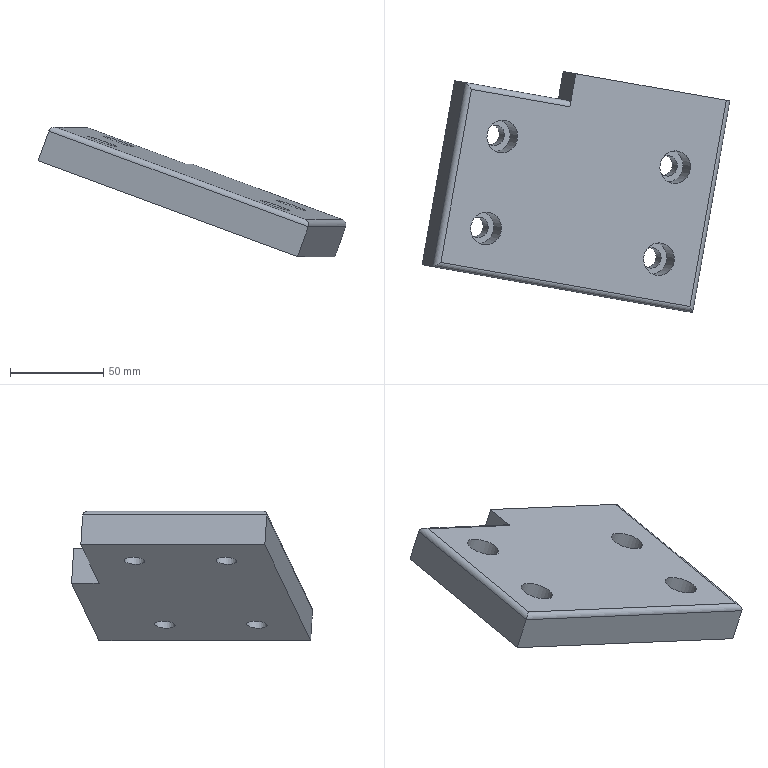Part | NX | features solid 2 | 1 solid | 24 faces | box 164.686 x 128.953 x 69.252 mm | volume 311600 mm3 | plane 12 | cylinder 12 | commonest cylinder face diameters 6 x4 11 x4 17.5 x4
STEP:
#1=CARTESIAN_POINT('',(-964.598,583.981,-183.949));
#2=VERTEX_POINT('',#1);
#3=CARTESIAN_POINT('',(-1020.123,593.771,-163.428));
#4=VERTEX_POINT('',#3);
#5=CARTESIAN_POINT('',(-834.947,561.12,-231.866));
#6=DIRECTION('',(-0.9254,0.1632,0.342));
#7=VECTOR('',#6,1000.);
#8=LINE('',#5,#7);
#9=EDGE_CURVE('',#2,#4,#8,.T.);
#10=ORIENTED_EDGE('',*,*,#9,.F.);
#11=CARTESIAN_POINT('',(-970.324,584.991,-199.924));
#12=VERTEX_POINT('',#11);
#13=CARTESIAN_POINT('',(-963.554,583.797,-181.036));
#14=DIRECTION('',(-0.3368,0.05939,-0.9397));
#15=VECTOR('',#14,1000.);
#16=LINE('',#13,#15);
#17=EDGE_CURVE('',#2,#12,#16,.T.);
#18=ORIENTED_EDGE('',*,*,#17,.T.);
#19=CARTESIAN_POINT('',(-1025.849,594.781,-179.402));
#20=VERTEX_POINT('',#19);
#21=CARTESIAN_POINT('',(-840.581,562.113,-247.875));
#22=DIRECTION('',(-0.9254,0.1632,0.342));
#23=VECTOR('',#22,1000.);
#24=LINE('',#21,#23);
#25=EDGE_CURVE('',#12,#20,#24,.T.);
#26=ORIENTED_EDGE('',*,*,#25,.T.);
#27=CARTESIAN_POINT('',(-1019.079,593.587,-160.515));
#28=DIRECTION('',(-0.3368,0.05939,-0.9397));
#29=VECTOR('',#28,1000.);
#30=LINE('',#27,#29);
#31=EDGE_CURVE('',#4,#20,#30,.T.);
#32=ORIENTED_EDGE('',*,*,#31,.F.);
#33=EDGE_LOOP('',(#10,#18,#26,#32));
#34=FACE_BOUND('',#33,.T.);
#35=CARTESIAN_POINT('',(-833.903,560.936,-228.953));
#36=DIRECTION('',(0.1736,0.9848,0.));
#37=DIRECTION('',(-0.9254,0.1632,0.342));
#38=AXIS2_PLACEMENT_3D('',#35,#36,#37);
#39=PLANE('',#38);
#40=ADVANCED_FACE('',(#34),#39,.T.);
#41=CARTESIAN_POINT('',(-898.675,470.814,-214.731));
#42=VERTEX_POINT('',#41);
#43=CARTESIAN_POINT('',(-878.706,584.067,-214.731));
#44=VERTEX_POINT('',#43);
#45=CARTESIAN_POINT('',(-880.625,573.185,-214.731));
#46=DIRECTION('',(-0.1736,-0.9848,0.));
#47=VECTOR('',#46,1000.);
#48=LINE('',#45,#47);
#49=EDGE_CURVE('',#42,#44,#48,.F.);
#50=ORIENTED_EDGE('',*,*,#49,.T.);
#51=CARTESIAN_POINT('',(-880.472,584.379,-210.886));
#52=VERTEX_POINT('',#51);
#53=CARTESIAN_POINT('',(-881.482,584.557,-213.705));
#54=DIRECTION('',(0.1736,0.9848,0.));
#55=DIRECTION('',(-0.9848,0.1736,0.));
#56=AXIS2_PLACEMENT_3D('',#53,#54,#55);
#57=CIRCLE('',#56,3.);
#58=EDGE_CURVE('',#44,#52,#57,.F.);
#59=ORIENTED_EDGE('',*,*,#58,.T.);
#60=CARTESIAN_POINT('',(-899.92,474.08,-210.886));
#61=VERTEX_POINT('',#60);
#62=CARTESIAN_POINT('',(-902.629,458.717,-210.886));
#63=DIRECTION('',(-0.1736,-0.9848,0.));
#64=VECTOR('',#63,1000.);
#65=LINE('',#62,#64);
#66=EDGE_CURVE('',#52,#61,#65,.T.);
#67=ORIENTED_EDGE('',*,*,#66,.T.);
#68=CARTESIAN_POINT('',(-900.931,474.258,-213.705));
#69=DIRECTION('',(0.7772,0.581,-0.2418));
#70=DIRECTION('',(0.5316,-0.8117,-0.2418));
#71=AXIS2_PLACEMENT_3D('',#68,#69,#70);
#72=ELLIPSE('',#71,4.243,3.);
#73=EDGE_CURVE('',#61,#42,#72,.T.);
#74=ORIENTED_EDGE('',*,*,#73,.T.);
#75=EDGE_LOOP('',(#50,#59,#67,#74));
#76=FACE_BOUND('',#75,.T.);
#77=CARTESIAN_POINT('',(-903.639,458.895,-213.705));
#78=DIRECTION('',(-0.1736,-0.9848,0.));
#79=DIRECTION('',(-0.9848,0.1736,0.));
#80=AXIS2_PLACEMENT_3D('',#77,#78,#79);
#81=CYLINDRICAL_SURFACE('',#80,3.);
#82=ADVANCED_FACE('',(#76),#81,.T.);
#83=CARTESIAN_POINT('',(-1016.857,590.149,-161.635));
#84=VERTEX_POINT('',#83);
#85=CARTESIAN_POINT('',(-964.108,580.848,-181.13));
#86=VERTEX_POINT('',#85);
#87=CARTESIAN_POINT('',(-834.365,557.971,-229.081));
#88=DIRECTION('',(-0.9254,0.1632,0.342));
#89=VECTOR('',#88,1000.);
#90=LINE('',#87,#89);
#91=EDGE_CURVE('',#84,#86,#90,.F.);
#92=ORIENTED_EDGE('',*,*,#91,.T.);
#93=CARTESIAN_POINT('',(-965.119,581.026,-183.949));
#94=DIRECTION('',(0.9254,-0.1632,-0.342));
#95=DIRECTION('',(-0.3467,0.,-0.938));
#96=AXIS2_PLACEMENT_3D('',#93,#94,#95);
#97=CIRCLE('',#96,3.);
#98=EDGE_CURVE('',#86,#2,#97,.F.);
#99=ORIENTED_EDGE('',*,*,#98,.T.);
#100=ORIENTED_EDGE('',*,*,#9,.T.);
#101=CARTESIAN_POINT('',(-1017.868,590.328,-164.454));
#102=DIRECTION('',(0.7772,0.581,-0.2418));
#103=DIRECTION('',(-0.5316,0.8117,0.2418));
#104=AXIS2_PLACEMENT_3D('',#101,#102,#103);
#105=ELLIPSE('',#104,4.243,3.);
#106=EDGE_CURVE('',#4,#84,#105,.T.);
#107=ORIENTED_EDGE('',*,*,#106,.T.);
#108=EDGE_LOOP('',(#92,#99,#100,#107));
#109=FACE_BOUND('',#108,.T.);
#110=CARTESIAN_POINT('',(-835.468,558.166,-231.866));
#111=DIRECTION('',(-0.9254,0.1632,0.342));
#112=DIRECTION('',(0.3368,-0.05939,0.9397));
#113=AXIS2_PLACEMENT_3D('',#110,#111,#112);
#114=CYLINDRICAL_SURFACE('',#113,3.);
#115=ADVANCED_FACE('',(#109),#114,.T.);
#116=CARTESIAN_POINT('',(-960.983,598.575,-181.13));
#117=VERTEX_POINT('',#116);
#118=CARTESIAN_POINT('',(-963.587,583.803,-181.13));
#119=DIRECTION('',(-0.1736,-0.9848,0.));
#120=VECTOR('',#119,1000.);
#121=LINE('',#118,#120);
#122=EDGE_CURVE('',#86,#117,#121,.F.);
#123=ORIENTED_EDGE('',*,*,#122,.F.);
#124=ORIENTED_EDGE('',*,*,#91,.F.);
#125=CARTESIAN_POINT('',(-1033.18,497.577,-161.635));
#126=VERTEX_POINT('',#125);
#127=CARTESIAN_POINT('',(-1035.889,482.214,-161.635));
#128=DIRECTION('',(-0.1736,-0.9848,0.));
#129=VECTOR('',#128,1000.);
#130=LINE('',#127,#129);
#131=EDGE_CURVE('',#126,#84,#130,.F.);
#132=ORIENTED_EDGE('',*,*,#131,.F.);
#133=CARTESIAN_POINT('',(-850.688,465.399,-229.081));
#134=DIRECTION('',(-0.9254,0.1632,0.342));
#135=VECTOR('',#134,1000.);
#136=LINE('',#133,#135);
#137=EDGE_CURVE('',#61,#126,#136,.T.);
#138=ORIENTED_EDGE('',*,*,#137,.F.);
#139=ORIENTED_EDGE('',*,*,#66,.F.);
#140=CARTESIAN_POINT('',(-831.332,575.714,-229.047));
#141=DIRECTION('',(0.9254,-0.1632,-0.342));
#142=VECTOR('',#141,1000.);
#143=LINE('',#140,#142);
#144=EDGE_CURVE('',#52,#117,#143,.F.);
#145=ORIENTED_EDGE('',*,*,#144,.T.);
#146=EDGE_LOOP('',(#123,#124,#132,#138,#139,#145));
#147=FACE_BOUND('',#146,.T.);
#148=CARTESIAN_POINT('',(-924.556,500.764,-200.368));
#149=VERTEX_POINT('',#148);
#150=CARTESIAN_POINT('',(-916.459,499.336,-203.361));
#151=DIRECTION('',(0.3368,-0.05939,0.9397));
#152=DIRECTION('',(-0.9254,0.1632,0.342));
#153=AXIS2_PLACEMENT_3D('',#150,#151,#152);
#154=CIRCLE('',#153,8.75);
#155=EDGE_CURVE('',#149,#149,#154,.T.);
#156=ORIENTED_EDGE('',*,*,#155,.F.);
#157=EDGE_LOOP('',(#156));
#158=FACE_BOUND('',#157,.T.);
#159=CARTESIAN_POINT('',(-915.874,550.004,-200.368));
#160=VERTEX_POINT('',#159);
#161=CARTESIAN_POINT('',(-907.777,548.576,-203.361));
#162=DIRECTION('',(0.3368,-0.05939,0.9397));
#163=DIRECTION('',(-0.9254,0.1632,0.342));
#164=AXIS2_PLACEMENT_3D('',#161,#162,#163);
#165=CIRCLE('',#164,8.75);
#166=EDGE_CURVE('',#160,#160,#165,.T.);
#167=ORIENTED_EDGE('',*,*,#166,.F.);
#168=EDGE_LOOP('',(#167));
#169=FACE_BOUND('',#168,.T.);
#170=CARTESIAN_POINT('',(-992.221,563.466,-172.152));
#171=VERTEX_POINT('',#170);
#172=CARTESIAN_POINT('',(-1000.318,564.894,-169.159));
#173=DIRECTION('',(-0.3368,0.05939,-0.9397));
#174=DIRECTION('',(0.9254,-0.1632,-0.342));
#175=AXIS2_PLACEMENT_3D('',#172,#173,#174);
#176=CIRCLE('',#175,8.75);
#177=EDGE_CURVE('',#171,#171,#176,.F.);
#178=ORIENTED_EDGE('',*,*,#177,.F.);
#179=EDGE_LOOP('',(#178));
#180=FACE_BOUND('',#179,.T.);
#181=CARTESIAN_POINT('',(-1000.903,514.226,-172.152));
#182=VERTEX_POINT('',#181);
#183=CARTESIAN_POINT('',(-1009.001,515.653,-169.159));
#184=DIRECTION('',(-0.3368,0.05939,-0.9397));
#185=DIRECTION('',(0.9254,-0.1632,-0.342));
#186=AXIS2_PLACEMENT_3D('',#183,#184,#185);
#187=CIRCLE('',#186,8.75);
#188=EDGE_CURVE('',#182,#182,#187,.F.);
#189=ORIENTED_EDGE('',*,*,#188,.F.);
#190=EDGE_LOOP('',(#189));
#191=FACE_BOUND('',#190,.T.);
#192=CARTESIAN_POINT('',(-853.397,450.036,-229.081));
#193=DIRECTION('',(0.3368,-0.05939,0.9397));
#194=DIRECTION('',(-0.9254,0.1632,0.342));
#195=AXIS2_PLACEMENT_3D('',#192,#193,#194);
#196=PLANE('',#195);
#197=ADVANCED_FACE('',(#147,#158,#169,#180,#191),#196,.T.);
#198=CARTESIAN_POINT('',(-884.432,585.077,-230.705));
#199=VERTEX_POINT('',#198);
#200=CARTESIAN_POINT('',(-877.662,583.883,-211.818));
#201=DIRECTION('',(0.3368,-0.05939,0.9397));
#202=VECTOR('',#201,1000.);
#203=LINE('',#200,#202);
#204=EDGE_CURVE('',#199,#44,#203,.T.);
#205=ORIENTED_EDGE('',*,*,#204,.T.);
#206=ORIENTED_EDGE('',*,*,#49,.F.);
#207=CARTESIAN_POINT('',(-904.401,471.824,-230.705));
#208=VERTEX_POINT('',#207);
#209=CARTESIAN_POINT('',(-904.772,471.889,-231.739));
#210=DIRECTION('',(0.3368,-0.05939,0.9397));
#211=VECTOR('',#210,1000.);
#212=LINE('',#209,#211);
#213=EDGE_CURVE('',#208,#42,#212,.T.);
#214=ORIENTED_EDGE('',*,*,#213,.F.);
#215=CARTESIAN_POINT('',(-906.572,459.514,-230.705));
#216=DIRECTION('',(0.1736,0.9848,0.));
#217=VECTOR('',#216,1000.);
#218=LINE('',#215,#217);
#219=EDGE_CURVE('',#208,#199,#218,.T.);
#220=ORIENTED_EDGE('',*,*,#219,.T.);
#221=EDGE_LOOP('',(#205,#206,#214,#220));
#222=FACE_BOUND('',#221,.T.);
#223=CARTESIAN_POINT('',(-886.721,574.26,-231.739));
#224=DIRECTION('',(0.9254,-0.1632,-0.342));
#225=DIRECTION('',(-0.1736,-0.9848,0.));
#226=AXIS2_PLACEMENT_3D('',#223,#224,#225);
#227=PLANE('',#226);
#228=ADVANCED_FACE('',(#222),#227,.T.);
#229=ORIENTED_EDGE('',*,*,#25,.F.);
#230=CARTESIAN_POINT('',(-967.719,599.763,-199.924));
#231=VERTEX_POINT('',#230);
#232=CARTESIAN_POINT('',(-970.324,584.991,-199.924));
#233=DIRECTION('',(0.1736,0.9848,0.));
#234=VECTOR('',#233,1000.);
#235=LINE('',#232,#234);
#236=EDGE_CURVE('',#12,#231,#235,.T.);
#237=ORIENTED_EDGE('',*,*,#236,.T.);
#238=CARTESIAN_POINT('',(-837.976,576.885,-247.875));
#239=DIRECTION('',(-0.9254,0.1632,0.342));
#240=VECTOR('',#239,1000.);
#241=LINE('',#238,#240);
#242=EDGE_CURVE('',#199,#231,#241,.T.);
#243=ORIENTED_EDGE('',*,*,#242,.F.);
#244=ORIENTED_EDGE('',*,*,#219,.F.);
#245=CARTESIAN_POINT('',(-1043.214,496.3,-179.402));
#246=VERTEX_POINT('',#245);
#247=CARTESIAN_POINT('',(-857.945,463.633,-247.875));
#248=DIRECTION('',(0.9254,-0.1632,-0.342));
#249=VECTOR('',#248,1000.);
#250=LINE('',#247,#249);
#251=EDGE_CURVE('',#246,#208,#250,.T.);
#252=ORIENTED_EDGE('',*,*,#251,.F.);
#253=CARTESIAN_POINT('',(-1028.176,581.585,-179.402));
#254=DIRECTION('',(0.1736,0.9848,0.));
#255=VECTOR('',#254,1000.);
#256=LINE('',#253,#255);
#257=EDGE_CURVE('',#246,#20,#256,.T.);
#258=ORIENTED_EDGE('',*,*,#257,.T.);
#259=EDGE_LOOP('',(#229,#237,#243,#244,#252,#258));
#260=FACE_BOUND('',#259,.T.);
#261=CARTESIAN_POINT('',(-928.285,501.421,-220.274));
#262=VERTEX_POINT('',#261);
#263=CARTESIAN_POINT('',(-923.196,500.524,-222.155));
#264=DIRECTION('',(0.3368,-0.05939,0.9397));
#265=DIRECTION('',(-0.9254,0.1632,0.342));
#266=AXIS2_PLACEMENT_3D('',#263,#264,#265);
#267=CIRCLE('',#266,5.5);
#268=EDGE_CURVE('',#262,#262,#267,.T.);
#269=ORIENTED_EDGE('',*,*,#268,.T.);
#270=EDGE_LOOP('',(#269));
#271=FACE_BOUND('',#270,.T.);
#272=CARTESIAN_POINT('',(-919.603,550.661,-220.274));
#273=VERTEX_POINT('',#272);
#274=CARTESIAN_POINT('',(-914.513,549.764,-222.155));
#275=DIRECTION('',(0.3368,-0.05939,0.9397));
#276=DIRECTION('',(-0.9254,0.1632,0.342));
#277=AXIS2_PLACEMENT_3D('',#274,#275,#276);
#278=CIRCLE('',#277,5.5);
#279=EDGE_CURVE('',#273,#273,#278,.T.);
#280=ORIENTED_EDGE('',*,*,#279,.T.);
#281=EDGE_LOOP('',(#280));
#282=FACE_BOUND('',#281,.T.);
#283=CARTESIAN_POINT('',(-1012.145,566.979,-186.072));
#284=VERTEX_POINT('',#283);
#285=CARTESIAN_POINT('',(-1007.055,566.082,-187.953));
#286=DIRECTION('',(0.3368,-0.05939,0.9397));
#287=DIRECTION('',(-0.9254,0.1632,0.342));
#288=AXIS2_PLACEMENT_3D('',#285,#286,#287);
#289=CIRCLE('',#288,5.5);
#290=EDGE_CURVE('',#284,#284,#289,.T.);
#291=ORIENTED_EDGE('',*,*,#290,.T.);
#292=EDGE_LOOP('',(#291));
#293=FACE_BOUND('',#292,.T.);
#294=CARTESIAN_POINT('',(-1020.827,517.739,-186.072));
#295=VERTEX_POINT('',#294);
#296=CARTESIAN_POINT('',(-1015.737,516.841,-187.953));
#297=DIRECTION('',(0.3368,-0.05939,0.9397));
#298=DIRECTION('',(-0.9254,0.1632,0.342));
#299=AXIS2_PLACEMENT_3D('',#296,#297,#298);
#300=CIRCLE('',#299,5.5);
#301=EDGE_CURVE('',#295,#295,#300,.T.);
#302=ORIENTED_EDGE('',*,*,#301,.T.);
#303=EDGE_LOOP('',(#302));
#304=FACE_BOUND('',#303,.T.);
#305=CARTESIAN_POINT('',(-839.877,566.102,-247.875));
#306=DIRECTION('',(-0.3368,0.05939,-0.9397));
#307=DIRECTION('',(-0.9254,0.1632,0.342));
#308=AXIS2_PLACEMENT_3D('',#305,#306,#307);
#309=PLANE('',#308);
#310=ADVANCED_FACE('',(#260,#271,#282,#293,#304),#309,.T.);
#311=ORIENTED_EDGE('',*,*,#31,.T.);
#312=ORIENTED_EDGE('',*,*,#257,.F.);
#313=CARTESIAN_POINT('',(-1037.488,495.291,-163.428));
#314=VERTEX_POINT('',#313);
#315=CARTESIAN_POINT('',(-1036.444,495.107,-160.515));
#316=DIRECTION('',(-0.3368,0.05939,-0.9397));
#317=VECTOR('',#316,1000.);
#318=LINE('',#315,#317);
#319=EDGE_CURVE('',#314,#246,#318,.T.);
#320=ORIENTED_EDGE('',*,*,#319,.F.);
#321=CARTESIAN_POINT('',(-1022.45,580.575,-163.428));
#322=DIRECTION('',(-0.1736,-0.9848,0.));
#323=VECTOR('',#322,1000.);
#324=LINE('',#321,#323);
#325=EDGE_CURVE('',#4,#314,#324,.T.);
#326=ORIENTED_EDGE('',*,*,#325,.F.);
#327=EDGE_LOOP('',(#311,#312,#320,#326));
#328=FACE_BOUND('',#327,.T.);
#329=CARTESIAN_POINT('',(-1021.406,580.391,-160.515));
#330=DIRECTION('',(-0.9254,0.1632,0.342));
#331=DIRECTION('',(-0.1736,-0.9848,0.));
#332=AXIS2_PLACEMENT_3D('',#329,#330,#331);
#333=PLANE('',#332);
#334=ADVANCED_FACE('',(#328),#333,.T.);
#335=ORIENTED_EDGE('',*,*,#319,.T.);
#336=ORIENTED_EDGE('',*,*,#251,.T.);
#337=ORIENTED_EDGE('',*,*,#213,.T.);
#338=CARTESIAN_POINT('',(-845.464,461.432,-234.397));
#339=DIRECTION('',(-0.9254,0.1632,0.342));
#340=VECTOR('',#339,1000.);
#341=LINE('',#338,#340);
#342=EDGE_CURVE('',#314,#42,#341,.F.);
#343=ORIENTED_EDGE('',*,*,#342,.F.);
#344=EDGE_LOOP('',(#335,#336,#337,#343));
#345=FACE_BOUND('',#344,.T.);
#346=CARTESIAN_POINT('',(-851.527,462.501,-251.311));
#347=DIRECTION('',(-0.1736,-0.9848,0.));
#348=DIRECTION('',(-0.9254,0.1632,0.342));
#349=AXIS2_PLACEMENT_3D('',#346,#347,#348);
#350=PLANE('',#349);
#351=ADVANCED_FACE('',(#345),#350,.T.);
#352=ORIENTED_EDGE('',*,*,#268,.F.);
#353=EDGE_LOOP('',(#352));
#354=FACE_BOUND('',#353,.T.);
#355=CARTESIAN_POINT('',(-925.591,500.946,-212.756));
#356=VERTEX_POINT('',#355);
#357=CARTESIAN_POINT('',(-920.501,500.048,-214.637));
#358=DIRECTION('',(0.3368,-0.05939,0.9397));
#359=DIRECTION('',(-0.9254,0.1632,0.342));
#360=AXIS2_PLACEMENT_3D('',#357,#358,#359);
#361=CIRCLE('',#360,5.5);
#362=EDGE_CURVE('',#356,#356,#361,.T.);
#363=ORIENTED_EDGE('',*,*,#362,.T.);
#364=EDGE_LOOP('',(#363));
#365=FACE_BOUND('',#364,.T.);
#366=CARTESIAN_POINT('',(-933.3,502.305,-250.346));
#367=DIRECTION('',(-0.3368,0.05939,-0.9397));
#368=DIRECTION('',(-0.9254,0.1632,0.342));
#369=AXIS2_PLACEMENT_3D('',#366,#367,#368);
#370=CYLINDRICAL_SURFACE('',#369,5.5);
#371=ADVANCED_FACE('',(#354,#365),#370,.F.);
#372=ORIENTED_EDGE('',*,*,#362,.F.);
#373=EDGE_LOOP('',(#372));
#374=FACE_BOUND('',#373,.T.);
#375=CARTESIAN_POINT('',(-928.598,501.476,-211.645));
#376=VERTEX_POINT('',#375);
#377=CARTESIAN_POINT('',(-920.501,500.048,-214.637));
#378=DIRECTION('',(0.3368,-0.05939,0.9397));
#379=DIRECTION('',(-0.9254,0.1632,0.342));
#380=AXIS2_PLACEMENT_3D('',#377,#378,#379);
#381=CIRCLE('',#380,8.75);
#382=EDGE_CURVE('',#376,#376,#381,.T.);
#383=ORIENTED_EDGE('',*,*,#382,.T.);
#384=EDGE_LOOP('',(#383));
#385=FACE_BOUND('',#384,.T.);
#386=CARTESIAN_POINT('',(-872.146,503.707,-231.738));
#387=DIRECTION('',(-0.3368,0.05939,-0.9397));
#388=DIRECTION('',(-0.9254,0.1632,0.342));
#389=AXIS2_PLACEMENT_3D('',#386,#387,#388);
#390=PLANE('',#389);
#391=ADVANCED_FACE('',(#374,#385),#390,.F.);
#392=ORIENTED_EDGE('',*,*,#382,.F.);
#393=EDGE_LOOP('',(#392));
#394=FACE_BOUND('',#393,.T.);
#395=ORIENTED_EDGE('',*,*,#155,.T.);
#396=EDGE_LOOP('',(#395));
#397=FACE_BOUND('',#396,.T.);
#398=CARTESIAN_POINT('',(-916.459,499.336,-203.361));
#399=DIRECTION('',(-0.3368,0.05939,-0.9397));
#400=DIRECTION('',(-0.9254,0.1632,0.342));
#401=AXIS2_PLACEMENT_3D('',#398,#399,#400);
#402=CYLINDRICAL_SURFACE('',#401,8.75);
#403=ADVANCED_FACE('',(#394,#397),#402,.F.);
#404=ORIENTED_EDGE('',*,*,#279,.F.);
#405=EDGE_LOOP('',(#404));
#406=FACE_BOUND('',#405,.T.);
#407=CARTESIAN_POINT('',(-916.908,550.186,-212.756));
#408=VERTEX_POINT('',#407);
#409=CARTESIAN_POINT('',(-911.818,549.289,-214.637));
#410=DIRECTION('',(0.3368,-0.05939,0.9397));
#411=DIRECTION('',(-0.9254,0.1632,0.342));
#412=AXIS2_PLACEMENT_3D('',#409,#410,#411);
#413=CIRCLE('',#412,5.5);
#414=EDGE_CURVE('',#408,#408,#413,.T.);
#415=ORIENTED_EDGE('',*,*,#414,.T.);
#416=EDGE_LOOP('',(#415));
#417=FACE_BOUND('',#416,.T.);
#418=CARTESIAN_POINT('',(-924.618,551.546,-250.346));
#419=DIRECTION('',(-0.3368,0.05939,-0.9397));
#420=DIRECTION('',(-0.9254,0.1632,0.342));
#421=AXIS2_PLACEMENT_3D('',#418,#419,#420);
#422=CYLINDRICAL_SURFACE('',#421,5.5);
#423=ADVANCED_FACE('',(#406,#417),#422,.F.);
#424=ORIENTED_EDGE('',*,*,#414,.F.);
#425=EDGE_LOOP('',(#424));
#426=FACE_BOUND('',#425,.T.);
#427=CARTESIAN_POINT('',(-919.916,550.717,-211.645));
#428=VERTEX_POINT('',#427);
#429=CARTESIAN_POINT('',(-911.818,549.289,-214.637));
#430=DIRECTION('',(0.3368,-0.05939,0.9397));
#431=DIRECTION('',(-0.9254,0.1632,0.342));
#432=AXIS2_PLACEMENT_3D('',#429,#430,#431);
#433=CIRCLE('',#432,8.75);
#434=EDGE_CURVE('',#428,#428,#433,.T.);
#435=ORIENTED_EDGE('',*,*,#434,.T.);
#436=EDGE_LOOP('',(#435));
#437=FACE_BOUND('',#436,.T.);
#438=CARTESIAN_POINT('',(-867.805,528.328,-231.738));
#439=DIRECTION('',(-0.3368,0.05939,-0.9397));
#440=DIRECTION('',(-0.9254,0.1632,0.342));
#441=AXIS2_PLACEMENT_3D('',#438,#439,#440);
#442=PLANE('',#441);
#443=ADVANCED_FACE('',(#426,#437),#442,.F.);
#444=ORIENTED_EDGE('',*,*,#434,.F.);
#445=EDGE_LOOP('',(#444));
#446=FACE_BOUND('',#445,.T.);
#447=ORIENTED_EDGE('',*,*,#166,.T.);
#448=EDGE_LOOP('',(#447));
#449=FACE_BOUND('',#448,.T.);
#450=CARTESIAN_POINT('',(-907.777,548.576,-203.361));
#451=DIRECTION('',(-0.3368,0.05939,-0.9397));
#452=DIRECTION('',(-0.9254,0.1632,0.342));
#453=AXIS2_PLACEMENT_3D('',#450,#451,#452);
#454=CYLINDRICAL_SURFACE('',#453,8.75);
#455=ADVANCED_FACE('',(#446,#449),#454,.F.);
#456=ORIENTED_EDGE('',*,*,#290,.F.);
#457=EDGE_LOOP('',(#456));
#458=FACE_BOUND('',#457,.T.);
#459=CARTESIAN_POINT('',(-1009.45,566.504,-178.554));
#460=VERTEX_POINT('',#459);
#461=CARTESIAN_POINT('',(-1004.36,565.606,-180.435));
#462=DIRECTION('',(0.3368,-0.05939,0.9397));
#463=DIRECTION('',(-0.9254,0.1632,0.342));
#464=AXIS2_PLACEMENT_3D('',#461,#462,#463);
#465=CIRCLE('',#464,5.5);
#466=EDGE_CURVE('',#460,#460,#465,.T.);
#467=ORIENTED_EDGE('',*,*,#466,.T.);
#468=EDGE_LOOP('',(#467));
#469=FACE_BOUND('',#468,.T.);
#470=CARTESIAN_POINT('',(-1017.159,567.863,-216.144));
#471=DIRECTION('',(-0.3368,0.05939,-0.9397));
#472=DIRECTION('',(-0.9254,0.1632,0.342));
#473=AXIS2_PLACEMENT_3D('',#470,#471,#472);
#474=CYLINDRICAL_SURFACE('',#473,5.5);
#475=ADVANCED_FACE('',(#458,#469),#474,.F.);
#476=ORIENTED_EDGE('',*,*,#466,.F.);
#477=EDGE_LOOP('',(#476));
#478=FACE_BOUND('',#477,.T.);
#479=CARTESIAN_POINT('',(-1012.458,567.034,-177.443));
#480=VERTEX_POINT('',#479);
#481=CARTESIAN_POINT('',(-1004.36,565.606,-180.435));
#482=DIRECTION('',(0.3368,-0.05939,0.9397));
#483=DIRECTION('',(-0.9254,0.1632,0.342));
#484=AXIS2_PLACEMENT_3D('',#481,#482,#483);
#485=CIRCLE('',#484,8.75);
#486=EDGE_CURVE('',#480,#480,#485,.T.);
#487=ORIENTED_EDGE('',*,*,#486,.T.);
#488=EDGE_LOOP('',(#487));
#489=FACE_BOUND('',#488,.T.);
#490=CARTESIAN_POINT('',(-1052.888,560.963,-163.334));
#491=DIRECTION('',(-0.3368,0.05939,-0.9397));
#492=DIRECTION('',(-0.9254,0.1632,0.342));
#493=AXIS2_PLACEMENT_3D('',#490,#491,#492);
#494=PLANE('',#493);
#495=ADVANCED_FACE('',(#478,#489),#494,.F.);
#496=ORIENTED_EDGE('',*,*,#486,.F.);
#497=EDGE_LOOP('',(#496));
#498=FACE_BOUND('',#497,.T.);
#499=ORIENTED_EDGE('',*,*,#177,.T.);
#500=EDGE_LOOP('',(#499));
#501=FACE_BOUND('',#500,.T.);
#502=CARTESIAN_POINT('',(-1000.318,564.894,-169.159));
#503=DIRECTION('',(-0.3368,0.05939,-0.9397));
#504=DIRECTION('',(-0.9254,0.1632,0.342));
#505=AXIS2_PLACEMENT_3D('',#502,#503,#504);
#506=CYLINDRICAL_SURFACE('',#505,8.75);
#507=ADVANCED_FACE('',(#498,#501),#506,.F.);
#508=ORIENTED_EDGE('',*,*,#301,.F.);
#509=EDGE_LOOP('',(#508));
#510=FACE_BOUND('',#509,.T.);
#511=CARTESIAN_POINT('',(-1018.132,517.263,-178.554));
#512=VERTEX_POINT('',#511);
#513=CARTESIAN_POINT('',(-1013.043,516.366,-180.435));
#514=DIRECTION('',(0.3368,-0.05939,0.9397));
#515=DIRECTION('',(-0.9254,0.1632,0.342));
#516=AXIS2_PLACEMENT_3D('',#513,#514,#515);
#517=CIRCLE('',#516,5.5);
#518=EDGE_CURVE('',#512,#512,#517,.T.);
#519=ORIENTED_EDGE('',*,*,#518,.T.);
#520=EDGE_LOOP('',(#519));
#521=FACE_BOUND('',#520,.T.);
#522=CARTESIAN_POINT('',(-1025.842,518.623,-216.144));
#523=DIRECTION('',(-0.3368,0.05939,-0.9397));
#524=DIRECTION('',(-0.9254,0.1632,0.342));
#525=AXIS2_PLACEMENT_3D('',#522,#523,#524);
#526=CYLINDRICAL_SURFACE('',#525,5.5);
#527=ADVANCED_FACE('',(#510,#521),#526,.F.);
#528=ORIENTED_EDGE('',*,*,#518,.F.);
#529=EDGE_LOOP('',(#528));
#530=FACE_BOUND('',#529,.T.);
#531=CARTESIAN_POINT('',(-1021.14,517.794,-177.443));
#532=VERTEX_POINT('',#531);
#533=CARTESIAN_POINT('',(-1013.043,516.366,-180.435));
#534=DIRECTION('',(0.3368,-0.05939,0.9397));
#535=DIRECTION('',(-0.9254,0.1632,0.342));
#536=AXIS2_PLACEMENT_3D('',#533,#534,#535);
#537=CIRCLE('',#536,8.75);
#538=EDGE_CURVE('',#532,#532,#537,.T.);
#539=ORIENTED_EDGE('',*,*,#538,.T.);
#540=EDGE_LOOP('',(#539));
#541=FACE_BOUND('',#540,.T.);
#542=CARTESIAN_POINT('',(-1010.959,528.184,-180.435));
#543=DIRECTION('',(-0.3368,0.05939,-0.9397));
#544=DIRECTION('',(-0.9254,0.1632,0.342));
#545=AXIS2_PLACEMENT_3D('',#542,#543,#544);
#546=PLANE('',#545);
#547=ADVANCED_FACE('',(#530,#541),#546,.F.);
#548=ORIENTED_EDGE('',*,*,#538,.F.);
#549=EDGE_LOOP('',(#548));
#550=FACE_BOUND('',#549,.T.);
#551=ORIENTED_EDGE('',*,*,#188,.T.);
#552=EDGE_LOOP('',(#551));
#553=FACE_BOUND('',#552,.T.);
#554=CARTESIAN_POINT('',(-1009.001,515.653,-169.159));
#555=DIRECTION('',(-0.3368,0.05939,-0.9397));
#556=DIRECTION('',(-0.9254,0.1632,0.342));
#557=AXIS2_PLACEMENT_3D('',#554,#555,#556);
#558=CYLINDRICAL_SURFACE('',#557,8.75);
#559=ADVANCED_FACE('',(#550,#553),#558,.F.);
#560=ORIENTED_EDGE('',*,*,#73,.F.);
#561=ORIENTED_EDGE('',*,*,#137,.T.);
#562=CARTESIAN_POINT('',(-1034.191,497.756,-164.454));
#563=DIRECTION('',(0.5316,-0.8117,-0.2418));
#564=DIRECTION('',(-0.7772,-0.581,0.2418));
#565=AXIS2_PLACEMENT_3D('',#562,#563,#564);
#566=ELLIPSE('',#565,4.243,3.);
#567=EDGE_CURVE('',#126,#314,#566,.T.);
#568=ORIENTED_EDGE('',*,*,#567,.T.);
#569=ORIENTED_EDGE('',*,*,#342,.T.);
#570=EDGE_LOOP('',(#560,#561,#568,#569));
#571=FACE_BOUND('',#570,.T.);
#572=CARTESIAN_POINT('',(-851.698,465.577,-231.9));
#573=DIRECTION('',(-0.9254,0.1632,0.342));
#574=DIRECTION('',(0.3368,-0.05939,0.9397));
#575=AXIS2_PLACEMENT_3D('',#572,#573,#574);
#576=CYLINDRICAL_SURFACE('',#575,3.);
#577=ADVANCED_FACE('',(#571),#576,.T.);
#578=ORIENTED_EDGE('',*,*,#106,.F.);
#579=ORIENTED_EDGE('',*,*,#325,.T.);
#580=ORIENTED_EDGE('',*,*,#567,.F.);
#581=ORIENTED_EDGE('',*,*,#131,.T.);
#582=EDGE_LOOP('',(#578,#579,#580,#581));
#583=FACE_BOUND('',#582,.T.);
#584=CARTESIAN_POINT('',(-1019.674,580.086,-164.454));
#585=DIRECTION('',(-0.1736,-0.9848,0.));
#586=DIRECTION('',(-0.9848,0.1736,0.));
#587=AXIS2_PLACEMENT_3D('',#584,#585,#586);
#588=CYLINDRICAL_SURFACE('',#587,3.);
#589=ADVANCED_FACE('',(#583),#588,.T.);
#590=ORIENTED_EDGE('',*,*,#17,.F.);
#591=ORIENTED_EDGE('',*,*,#98,.F.);
#592=ORIENTED_EDGE('',*,*,#122,.T.);
#593=CARTESIAN_POINT('',(-960.949,598.569,-181.036));
#594=DIRECTION('',(-0.3368,0.05939,-0.9397));
#595=VECTOR('',#594,1000.);
#596=LINE('',#593,#595);
#597=EDGE_CURVE('',#117,#231,#596,.T.);
#598=ORIENTED_EDGE('',*,*,#597,.T.);
#599=ORIENTED_EDGE('',*,*,#236,.F.);
#600=EDGE_LOOP('',(#590,#591,#592,#598,#599));
#601=FACE_BOUND('',#600,.T.);
#602=CARTESIAN_POINT('',(-963.554,583.797,-181.036));
#603=DIRECTION('',(0.9254,-0.1632,-0.342));
#604=DIRECTION('',(-0.3467,0.,-0.938));
#605=AXIS2_PLACEMENT_3D('',#602,#603,#604);
#606=PLANE('',#605);
#607=ADVANCED_FACE('',(#601),#606,.F.);
#608=ORIENTED_EDGE('',*,*,#58,.F.);
#609=ORIENTED_EDGE('',*,*,#204,.F.);
#610=ORIENTED_EDGE('',*,*,#242,.T.);
#611=ORIENTED_EDGE('',*,*,#597,.F.);
#612=ORIENTED_EDGE('',*,*,#144,.F.);
#613=EDGE_LOOP('',(#608,#609,#610,#611,#612));
#614=FACE_BOUND('',#613,.T.);
#615=CARTESIAN_POINT('',(-831.298,575.708,-228.953));
#616=DIRECTION('',(0.1736,0.9848,0.));
#617=DIRECTION('',(-0.9254,0.1632,0.342));
#618=AXIS2_PLACEMENT_3D('',#615,#616,#617);
#619=PLANE('',#618);
#620=ADVANCED_FACE('',(#614),#619,.T.);
#621=CLOSED_SHELL('',(#40,#82,#115,#197,#228,#310,#334,#351,#371,#391,#403,#423,#443,#455,#475,#495,#507,#527,#547,#559,#577,#589,#607,#620));
#622=MANIFOLD_SOLID_BREP('',#621);
#623=(LENGTH_UNIT()NAMED_UNIT(*)SI_UNIT(.MILLI.,.METRE.));
#624=UNCERTAINTY_MEASURE_WITH_UNIT(LENGTH_MEASURE(0.00001),#623,'','');
#625=(NAMED_UNIT(*)PLANE_ANGLE_UNIT()SI_UNIT($,.RADIAN.));
#626=(NAMED_UNIT(*)SI_UNIT($,.STERADIAN.)SOLID_ANGLE_UNIT());
#627=(GEOMETRIC_REPRESENTATION_CONTEXT(3)GLOBAL_UNCERTAINTY_ASSIGNED_CONTEXT((#624))GLOBAL_UNIT_ASSIGNED_CONTEXT((#623,#625,#626))REPRESENTATION_CONTEXT('',''));
#628=ADVANCED_BREP_SHAPE_REPRESENTATION('',(#622),#627);